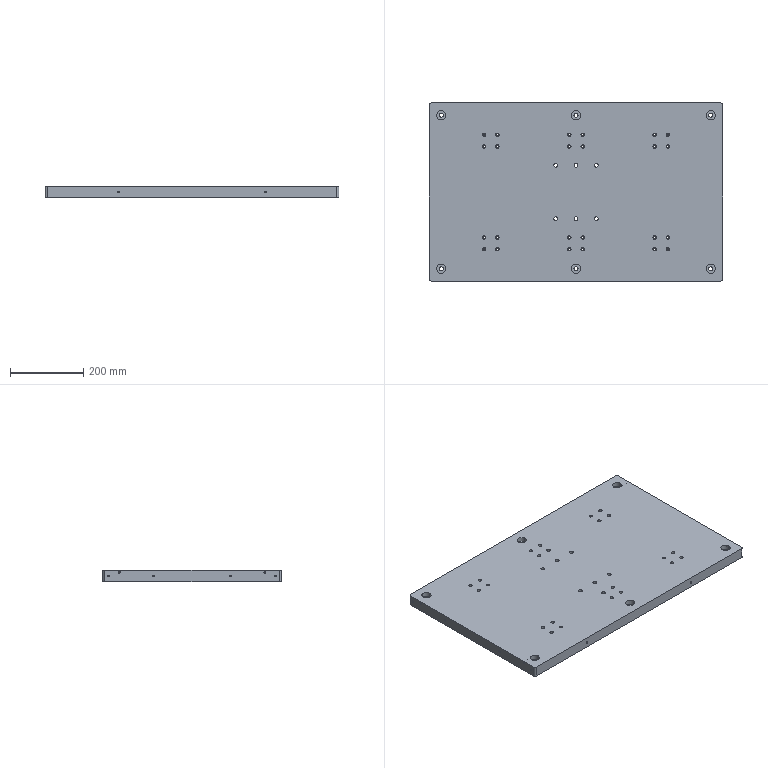NC program | Mastercam | posted with a generic post | part box 800 x 485 x 30 mm
Lines 1 to 760 of 3510:
%
O0000()
(MATERIAL - ALUMINUM MM - 2024)
( T20 | 20 FEM | H20 | XY STOCK TO LEAVE - .1 | Z STOCK TO LEAVE - .05 )
( T7 | 4 CHM | H7 )
( T1 | 11 DR | H1 | XY STOCK TO LEAVE - 0. | Z STOCK TO LEAVE - .05 )
( T14 | 10.5 DR | H14 )
( T9 | 10 FEM | H9 | XY STOCK TO LEAVE - .05 | Z STOCK TO LEAVE - .05 )
( T10 | 10 FEM | H10 | XY STOCK TO LEAVE - -.03 | Z STOCK TO LEAVE - 0. )
( T18 | 5.1 DR | H18 )
N100 G21
N110 G0 G17 G40 G49 G80 G90
( ?X )
N120 T20 M6
N130 G0 G90 G54 X-415. Y252.6 A0. S5000 M3
N140 G43 H20 Z50. M8
N150 Z1.
N160 G1 Z-.998 F600.
N170 X-395. F4000.
N180 X395.
N190 X415.
N200 Z-1.996 F600.
N210 X395. F4000.
N220 X-395.
N230 X-415.
N240 Z-2.994 F600.
N250 X-395. F4000.
N260 X395.
N270 X415.
N280 Z-3.992 F600.
N290 X395. F4000.
N300 X-395.
N310 X-415.
N320 Z-4.99 F600.
N330 X-395. F4000.
N340 X395.
N350 X415.
N360 Z-5.988 F600.
N370 X395. F4000.
N380 X-395.
N390 X-415.
N400 Z-6.986 F600.
N410 X-395. F4000.
N420 X395.
N430 X415.
N440 Z-7.984 F600.
N450 X395. F4000.
N460 X-395.
N470 X-415.
N480 Z-8.982 F600.
N490 X-395. F4000.
N500 X395.
N510 X415.
N520 Z-9.98 F600.
N530 X395. F4000.
N540 X-395.
N550 X-415.
N560 Z-10.978 F600.
N570 X-395. F4000.
N580 X395.
N590 X415.
N600 Z-11.976 F600.
N610 X395. F4000.
N620 X-395.
N630 X-415.
N640 Z-12.974 F600.
N650 X-395. F4000.
N660 X395.
N670 X415.
N680 Z-13.972 F600.
N690 X395. F4000.
N700 X-395.
N710 X-415.
N720 Z-14.97 F600.
N730 X-395. F4000.
N740 X395.
N750 X415.
N760 Z-15.968 F600.
N770 X395. F4000.
N780 X-395.
N790 X-415.
N800 Z-16.966 F600.
N810 X-395. F4000.
N820 X395.
N830 X415.
N840 Z-17.964 F600.
N850 X395. F4000.
N860 X-395.
N870 X-415.
N880 Z-18.962 F600.
N890 X-395. F4000.
N900 X395.
N910 X415.
N920 Z-19.96 F600.
N930 X395. F4000.
N940 X-395.
N950 X-415.
N960 Z-20.958 F600.
N970 X-395. F4000.
N980 X395.
N990 X415.
N1000 Z-21.956 F600.
N1010 X395. F4000.
N1020 X-395.
N1030 X-415.
N1040 Z-22.954 F600.
N1050 X-395. F4000.
N1060 X395.
N1070 X415.
N1080 Z-23.952 F600.
N1090 X395. F4000.
N1100 X-395.
N1110 X-415.
N1120 Z-24.95 F600.
N1130 X-395. F4000.
N1140 X395.
N1150 X415.
N1160 G0 Z50.
N1170 Y-252.6
N1180 Z1.
N1190 G1 Z-.998 F600.
N1200 X395. F4000.
N1210 X-395.
N1220 X-415.
N1230 Z-1.996 F600.
N1240 X-395. F4000.
N1250 X395.
N1260 X415.
N1270 Z-2.994 F600.
N1280 X395. F4000.
N1290 X-395.
N1300 X-415.
N1310 Z-3.992 F600.
N1320 X-395. F4000.
N1330 X395.
N1340 X415.
N1350 Z-4.99 F600.
N1360 X395. F4000.
N1370 X-395.
N1380 X-415.
N1390 Z-5.988 F600.
N1400 X-395. F4000.
N1410 X395.
N1420 X415.
N1430 Z-6.986 F600.
N1440 X395. F4000.
N1450 X-395.
N1460 X-415.
N1470 Z-7.984 F600.
N1480 X-395. F4000.
N1490 X395.
N1500 X415.
N1510 Z-8.982 F600.
N1520 X395. F4000.
N1530 X-395.
N1540 X-415.
N1550 Z-9.98 F600.
N1560 X-395. F4000.
N1570 X395.
N1580 X415.
N1590 Z-10.978 F600.
N1600 X395. F4000.
N1610 X-395.
N1620 X-415.
N1630 Z-11.976 F600.
N1640 X-395. F4000.
N1650 X395.
N1660 X415.
N1670 Z-12.974 F600.
N1680 X395. F4000.
N1690 X-395.
N1700 X-415.
N1710 Z-13.972 F600.
N1720 X-395. F4000.
N1730 X395.
N1740 X415.
N1750 Z-14.97 F600.
N1760 X395. F4000.
N1770 X-395.
N1780 X-415.
N1790 Z-15.968 F600.
N1800 X-395. F4000.
N1810 X395.
N1820 X415.
N1830 Z-16.966 F600.
N1840 X395. F4000.
N1850 X-395.
N1860 X-415.
N1870 Z-17.964 F600.
N1880 X-395. F4000.
N1890 X395.
N1900 X415.
N1910 Z-18.962 F600.
N1920 X395. F4000.
N1930 X-395.
N1940 X-415.
N1950 Z-19.96 F600.
N1960 X-395. F4000.
N1970 X395.
N1980 X415.
N1990 Z-20.958 F600.
N2000 X395. F4000.
N2010 X-395.
N2020 X-415.
N2030 Z-21.956 F600.
N2040 X-395. F4000.
N2050 X395.
N2060 X415.
N2070 Z-22.954 F600.
N2080 X395. F4000.
N2090 X-395.
N2100 X-415.
N2110 Z-23.952 F600.
N2120 X-395. F4000.
N2130 X395.
N2140 X415.
N2150 Z-24.95 F600.
N2160 X395. F4000.
N2170 X-395.
N2180 X-415.
N2190 G0 Z50.
N2200 Y252.53
N2210 Z1.
N2220 G1 Z-24.95 F600.
N2230 X-395. F1000.
N2240 X395.
N2250 X415.
N2260 G0 Z50.
N2270 X-415. Y252.5
N2280 Z1.
N2290 G1 Z-24.95 F600.
N2300 X-395. F1000.
N2310 X395.
N2320 X415.
N2330 G0 Z50.
N2340 Y-252.53
N2350 Z1.
N2360 G1 Z-24.95 F600.
N2370 X395. F1000.
N2380 X-395.
N2390 X-415.
N2400 G0 Z50.
N2410 X415. Y-252.5
N2420 Z1.
N2430 G1 Z-24.95 F600.
N2440 X395. F1000.
N2450 X-395.
N2460 X-415.
N2470 G0 Z50.
N2480 M5
N2490 G91 G28 Z0. M9
N2500 A0.
N2510 M01
N2520 T7 M6
N2530 G0 G90 G17 G54 X-405. Y243.15 A0. S6500 M3
N2540 G43 H7 Z50. M8
N2550 Z1.
N2560 G1 Z-.75 F600.
N2570 X-395. F1000.
N2580 X395.
N2590 X405.
N2600 G0 Z50.
N2610 Y-243.15
N2620 Z1.
N2630 G1 Z-.75 F600.
N2640 X395. F1000.
N2650 X-395.
N2660 X-405.
N2670 G0 Z50.
N2680 M5
N2690 G91 G28 Z0. M9
N2700 A0.
N2710 M01
( CCL,CY )
M00
N2720 T20 M6
N2730 G0 G90 G17 G54 X-393. Y-256.6 A0. S5000 M3
N2740 G43 H20 Z50. M8
N2750 Z1.
N2760 G1 Z-.998 F600.
N2770 Y-254.6 F4000.
N2780 G3 X-395. Y-252.6 I-2. J0.
N2790 G2 X-410.1 Y-237.5 I0. J15.1
N2800 G1 Y237.5
N2810 G2 X-395. Y252.6 I15.1 J0.
N2820 G3 X-393. Y254.6 I0. J2.
N2830 G1 Y256.6
N2840 Z-1.996 F600.
N2850 Y254.6 F4000.
N2860 G2 X-395. Y252.6 I-2. J0.
N2870 G3 X-410.1 Y237.5 I0. J-15.1
N2880 G1 Y-237.5
N2890 G3 X-395. Y-252.6 I15.1 J0.
N2900 G2 X-393. Y-254.6 I0. J-2.
N2910 G1 Y-256.6
N2920 Z-2.994 F600.
N2930 Y-254.6 F4000.
N2940 G3 X-395. Y-252.6 I-2. J0.
N2950 G2 X-410.1 Y-237.5 I0. J15.1
N2960 G1 Y237.5
N2970 G2 X-395. Y252.6 I15.1 J0.
N2980 G3 X-393. Y254.6 I0. J2.
N2990 G1 Y256.6
N3000 Z-3.992 F600.
N3010 Y254.6 F4000.
N3020 G2 X-395. Y252.6 I-2. J0.
N3030 G3 X-410.1 Y237.5 I0. J-15.1
N3040 G1 Y-237.5
N3050 G3 X-395. Y-252.6 I15.1 J0.
N3060 G2 X-393. Y-254.6 I0. J-2.
N3070 G1 Y-256.6
N3080 Z-4.99 F600.
N3090 Y-254.6 F4000.
N3100 G3 X-395. Y-252.6 I-2. J0.
N3110 G2 X-410.1 Y-237.5 I0. J15.1
N3120 G1 Y237.5
N3130 G2 X-395. Y252.6 I15.1 J0.
N3140 G3 X-393. Y254.6 I0. J2.
N3150 G1 Y256.6
N3160 Z-5.988 F600.
N3170 Y254.6 F4000.
N3180 G2 X-395. Y252.6 I-2. J0.
N3190 G3 X-410.1 Y237.5 I0. J-15.1
N3200 G1 Y-237.5
N3210 G3 X-395. Y-252.6 I15.1 J0.
N3220 G2 X-393. Y-254.6 I0. J-2.
N3230 G1 Y-256.6
N3240 Z-6.986 F600.
N3250 Y-254.6 F4000.
N3260 G3 X-395. Y-252.6 I-2. J0.
N3270 G2 X-410.1 Y-237.5 I0. J15.1
N3280 G1 Y237.5
N3290 G2 X-395. Y252.6 I15.1 J0.
N3300 G3 X-393. Y254.6 I0. J2.
N3310 G1 Y256.6
N3320 Z-7.984 F600.
N3330 Y254.6 F4000.
N3340 G2 X-395. Y252.6 I-2. J0.
N3350 G3 X-410.1 Y237.5 I0. J-15.1
N3360 G1 Y-237.5
N3370 G3 X-395. Y-252.6 I15.1 J0.
N3380 G2 X-393. Y-254.6 I0. J-2.
N3390 G1 Y-256.6
N3400 Z-8.982 F600.
N3410 Y-254.6 F4000.
N3420 G3 X-395. Y-252.6 I-2. J0.
N3430 G2 X-410.1 Y-237.5 I0. J15.1
N3440 G1 Y237.5
N3450 G2 X-395. Y252.6 I15.1 J0.
N3460 G3 X-393. Y254.6 I0. J2.
N3470 G1 Y256.6
N3480 Z-9.98 F600.
N3490 Y254.6 F4000.
N3500 G2 X-395. Y252.6 I-2. J0.
N3510 G3 X-410.1 Y237.5 I0. J-15.1
N3520 G1 Y-237.5
N3530 G3 X-395. Y-252.6 I15.1 J0.
N3540 G2 X-393. Y-254.6 I0. J-2.
N3550 G1 Y-256.6
N3560 Z-10.978 F600.
N3570 Y-254.6 F4000.
N3580 G3 X-395. Y-252.6 I-2. J0.
N3590 G2 X-410.1 Y-237.5 I0. J15.1
N3600 G1 Y237.5
N3610 G2 X-395. Y252.6 I15.1 J0.
N3620 G3 X-393. Y254.6 I0. J2.
N3630 G1 Y256.6
N3640 Z-11.976 F600.
N3650 Y254.6 F4000.
N3660 G2 X-395. Y252.6 I-2. J0.
N3670 G3 X-410.1 Y237.5 I0. J-15.1
N3680 G1 Y-237.5
N3690 G3 X-395. Y-252.6 I15.1 J0.
N3700 G2 X-393. Y-254.6 I0. J-2.
N3710 G1 Y-256.6
N3720 Z-12.974 F600.
N3730 Y-254.6 F4000.
N3740 G3 X-395. Y-252.6 I-2. J0.
N3750 G2 X-410.1 Y-237.5 I0. J15.1
N3760 G1 Y237.5
N3770 G2 X-395. Y252.6 I15.1 J0.
N3780 G3 X-393. Y254.6 I0. J2.
N3790 G1 Y256.6
N3800 Z-13.972 F600.
N3810 Y254.6 F4000.
N3820 G2 X-395. Y252.6 I-2. J0.
N3830 G3 X-410.1 Y237.5 I0. J-15.1
N3840 G1 Y-237.5
N3850 G3 X-395. Y-252.6 I15.1 J0.
N3860 G2 X-393. Y-254.6 I0. J-2.
N3870 G1 Y-256.6
N3880 Z-14.97 F600.
N3890 Y-254.6 F4000.
N3900 G3 X-395. Y-252.6 I-2. J0.
N3910 G2 X-410.1 Y-237.5 I0. J15.1
N3920 G1 Y237.5
N3930 G2 X-395. Y252.6 I15.1 J0.
N3940 G3 X-393. Y254.6 I0. J2.
N3950 G1 Y256.6
N3960 Z-15.968 F600.
N3970 Y254.6 F4000.
N3980 G2 X-395. Y252.6 I-2. J0.
N3990 G3 X-410.1 Y237.5 I0. J-15.1
N4000 G1 Y-237.5
N4010 G3 X-395. Y-252.6 I15.1 J0.
N4020 G2 X-393. Y-254.6 I0. J-2.
N4030 G1 Y-256.6
N4040 Z-16.966 F600.
N4050 Y-254.6 F4000.
N4060 G3 X-395. Y-252.6 I-2. J0.
N4070 G2 X-410.1 Y-237.5 I0. J15.1
N4080 G1 Y237.5
N4090 G2 X-395. Y252.6 I15.1 J0.
N4100 G3 X-393. Y254.6 I0. J2.
N4110 G1 Y256.6
N4120 Z-17.964 F600.
N4130 Y254.6 F4000.
N4140 G2 X-395. Y252.6 I-2. J0.
N4150 G3 X-410.1 Y237.5 I0. J-15.1
N4160 G1 Y-237.5
N4170 G3 X-395. Y-252.6 I15.1 J0.
N4180 G2 X-393. Y-254.6 I0. J-2.
N4190 G1 Y-256.6
N4200 Z-18.962 F600.
N4210 Y-254.6 F4000.
N4220 G3 X-395. Y-252.6 I-2. J0.
N4230 G2 X-410.1 Y-237.5 I0. J15.1
N4240 G1 Y237.5
N4250 G2 X-395. Y252.6 I15.1 J0.
N4260 G3 X-393. Y254.6 I0. J2.
N4270 G1 Y256.6
N4280 Z-19.96 F600.
N4290 Y254.6 F4000.
N4300 G2 X-395. Y252.6 I-2. J0.
N4310 G3 X-410.1 Y237.5 I0. J-15.1
N4320 G1 Y-237.5
N4330 G3 X-395. Y-252.6 I15.1 J0.
N4340 G2 X-393. Y-254.6 I0. J-2.
N4350 G1 Y-256.6
N4360 Z-20.958 F600.
N4370 Y-254.6 F4000.
N4380 G3 X-395. Y-252.6 I-2. J0.
N4390 G2 X-410.1 Y-237.5 I0. J15.1
N4400 G1 Y237.5
N4410 G2 X-395. Y252.6 I15.1 J0.
N4420 G3 X-393. Y254.6 I0. J2.
N4430 G1 Y256.6
N4440 Z-21.956 F600.
N4450 Y254.6 F4000.
N4460 G2 X-395. Y252.6 I-2. J0.
N4470 G3 X-410.1 Y237.5 I0. J-15.1
N4480 G1 Y-237.5
N4490 G3 X-395. Y-252.6 I15.1 J0.
N4500 G2 X-393. Y-254.6 I0. J-2.
N4510 G1 Y-256.6
N4520 Z-22.954 F600.
N4530 Y-254.6 F4000.
N4540 G3 X-395. Y-252.6 I-2. J0.
N4550 G2 X-410.1 Y-237.5 I0. J15.1
N4560 G1 Y237.5
N4570 G2 X-395. Y252.6 I15.1 J0.
N4580 G3 X-393. Y254.6 I0. J2.
N4590 G1 Y256.6
N4600 Z-23.952 F600.
N4610 Y254.6 F4000.
N4620 G2 X-395. Y252.6 I-2. J0.
N4630 G3 X-410.1 Y237.5 I0. J-15.1
N4640 G1 Y-237.5
N4650 G3 X-395. Y-252.6 I15.1 J0.
N4660 G2 X-393. Y-254.6 I0. J-2.
N4670 G1 Y-256.6
N4680 Z-24.95 F600.
N4690 Y-254.6 F4000.
N4700 G3 X-395. Y-252.6 I-2. J0.
N4710 G2 X-410.1 Y-237.5 I0. J15.1
N4720 G1 Y237.5
N4730 G2 X-395. Y252.6 I15.1 J0.
N4740 G3 X-393. Y254.6 I0. J2.
N4750 G1 Y256.6
N4760 G0 Z50.
N4770 X393.
N4780 Z1.
N4790 G1 Z-.998 F600.
N4800 Y254.6 F4000.
N4810 G3 X395. Y252.6 I2. J0.
N4820 G2 X410.1 Y237.5 I0. J-15.1
N4830 G1 Y-237.5
N4840 G2 X395. Y-252.6 I-15.1 J0.
N4850 G3 X393. Y-254.6 I0. J-2.
N4860 G1 Y-256.6
N4870 Z-1.996 F600.
N4880 Y-254.6 F4000.
N4890 G2 X395. Y-252.6 I2. J0.
N4900 G3 X410.1 Y-237.5 I0. J15.1
N4910 G1 Y237.5
N4920 G3 X395. Y252.6 I-15.1 J0.
N4930 G2 X393. Y254.6 I0. J2.
N4940 G1 Y256.6
N4950 Z-2.994 F600.
N4960 Y254.6 F4000.
N4970 G3 X395. Y252.6 I2. J0.
N4980 G2 X410.1 Y237.5 I0. J-15.1
N4990 G1 Y-237.5
N5000 G2 X395. Y-252.6 I-15.1 J0.
N5010 G3 X393. Y-254.6 I0. J-2.
N5020 G1 Y-256.6
N5030 Z-3.992 F600.
N5040 Y-254.6 F4000.
N5050 G2 X395. Y-252.6 I2. J0.
N5060 G3 X410.1 Y-237.5 I0. J15.1
N5070 G1 Y237.5
N5080 G3 X395. Y252.6 I-15.1 J0.
N5090 G2 X393. Y254.6 I0. J2.
N5100 G1 Y256.6
N5110 Z-4.99 F600.
N5120 Y254.6 F4000.
N5130 G3 X395. Y252.6 I2. J0.
N5140 G2 X410.1 Y237.5 I0. J-15.1
N5150 G1 Y-237.5
N5160 G2 X395. Y-252.6 I-15.1 J0.
N5170 G3 X393. Y-254.6 I0. J-2.
N5180 G1 Y-256.6
N5190 Z-5.988 F600.
N5200 Y-254.6 F4000.
N5210 G2 X395. Y-252.6 I2. J0.
N5220 G3 X410.1 Y-237.5 I0. J15.1
N5230 G1 Y237.5
N5240 G3 X395. Y252.6 I-15.1 J0.
N5250 G2 X393. Y254.6 I0. J2.
N5260 G1 Y256.6
N5270 Z-6.986 F600.
N5280 Y254.6 F4000.
N5290 G3 X395. Y252.6 I2. J0.
N5300 G2 X410.1 Y237.5 I0. J-15.1
N5310 G1 Y-237.5
N5320 G2 X395. Y-252.6 I-15.1 J0.
N5330 G3 X393. Y-254.6 I0. J-2.
N5340 G1 Y-256.6
N5350 Z-7.984 F600.
N5360 Y-254.6 F4000.
N5370 G2 X395. Y-252.6 I2. J0.
N5380 G3 X410.1 Y-237.5 I0. J15.1
N5390 G1 Y237.5
N5400 G3 X395. Y252.6 I-15.1 J0.
N5410 G2 X393. Y254.6 I0. J2.
N5420 G1 Y256.6
N5430 Z-8.982 F600.
N5440 Y254.6 F4000.
N5450 G3 X395. Y252.6 I2. J0.
N5460 G2 X410.1 Y237.5 I0. J-15.1
N5470 G1 Y-237.5
N5480 G2 X395. Y-252.6 I-15.1 J0.
N5490 G3 X393. Y-254.6 I0. J-2.
N5500 G1 Y-256.6
N5510 Z-9.98 F600.
N5520 Y-254.6 F4000.
N5530 G2 X395. Y-252.6 I2. J0.
N5540 G3 X410.1 Y-237.5 I0. J15.1
N5550 G1 Y237.5
N5560 G3 X395. Y252.6 I-15.1 J0.
N5570 G2 X393. Y254.6 I0. J2.
N5580 G1 Y256.6
N5590 Z-10.978 F600.
N5600 Y254.6 F4000.
N5610 G3 X395. Y252.6 I2. J0.
N5620 G2 X410.1 Y237.5 I0. J-15.1
N5630 G1 Y-237.5
N5640 G2 X395. Y-252.6 I-15.1 J0.
N5650 G3 X393. Y-254.6 I0. J-2.
N5660 G1 Y-256.6
N5670 Z-11.976 F600.
N5680 Y-254.6 F4000.
N5690 G2 X395. Y-252.6 I2. J0.
N5700 G3 X410.1 Y-237.5 I0. J15.1
N5710 G1 Y237.5
N5720 G3 X395. Y252.6 I-15.1 J0.
N5730 G2 X393. Y254.6 I0. J2.
N5740 G1 Y256.6
N5750 Z-12.974 F600.
N5760 Y254.6 F4000.
N5770 G3 X395. Y252.6 I2. J0.
N5780 G2 X410.1 Y237.5 I0. J-15.1
N5790 G1 Y-237.5
N5800 G2 X395. Y-252.6 I-15.1 J0.
N5810 G3 X393. Y-254.6 I0. J-2.
N5820 G1 Y-256.6
N5830 Z-13.972 F600.
N5840 Y-254.6 F4000.
N5850 G2 X395. Y-252.6 I2. J0.
N5860 G3 X410.1 Y-237.5 I0. J15.1
N5870 G1 Y237.5
N5880 G3 X395. Y252.6 I-15.1 J0.
N5890 G2 X393. Y254.6 I0. J2.
N5900 G1 Y256.6
N5910 Z-14.97 F600.
N5920 Y254.6 F4000.
N5930 G3 X395. Y252.6 I2. J0.
N5940 G2 X410.1 Y237.5 I0. J-15.1
N5950 G1 Y-237.5
N5960 G2 X395. Y-252.6 I-15.1 J0.
N5970 G3 X393. Y-254.6 I0. J-2.
N5980 G1 Y-256.6
N5990 Z-15.968 F600.
N6000 Y-254.6 F4000.
N6010 G2 X395. Y-252.6 I2. J0.
N6020 G3 X410.1 Y-237.5 I0. J15.1
N6030 G1 Y237.5
N6040 G3 X395. Y252.6 I-15.1 J0.
N6050 G2 X393. Y254.6 I0. J2.
N6060 G1 Y256.6
N6070 Z-16.966 F600.
N6080 Y254.6 F4000.
N6090 G3 X395. Y252.6 I2. J0.
N6100 G2 X410.1 Y237.5 I0. J-15.1
N6110 G1 Y-237.5
N6120 G2 X395. Y-252.6 I-15.1 J0.
N6130 G3 X393. Y-254.6 I0. J-2.
N6140 G1 Y-256.6
N6150 Z-17.964 F600.
N6160 Y-254.6 F4000.
N6170 G2 X395. Y-252.6 I2. J0.
N6180 G3 X410.1 Y-237.5 I0. J15.1
N6190 G1 Y237.5
N6200 G3 X395. Y252.6 I-15.1 J0.
N6210 G2 X393. Y254.6 I0. J2.
N6220 G1 Y256.6
N6230 Z-18.962 F600.
N6240 Y254.6 F4000.
N6250 G3 X395. Y252.6 I2. J0.
N6260 G2 X410.1 Y237.5 I0. J-15.1
N6270 G1 Y-237.5
N6280 G2 X395. Y-252.6 I-15.1 J0.
N6290 G3 X393. Y-254.6 I0. J-2.
N6300 G1 Y-256.6
N6310 Z-19.96 F600.
N6320 Y-254.6 F4000.
N6330 G2 X395. Y-252.6 I2. J0.
N6340 G3 X410.1 Y-237.5 I0. J15.1
N6350 G1 Y237.5
N6360 G3 X395. Y252.6 I-15.1 J0.
N6370 G2 X393. Y254.6 I0. J2.
N6380 G1 Y256.6
N6390 Z-20.958 F600.
N6400 Y254.6 F4000.
N6410 G3 X395. Y252.6 I2. J0.
N6420 G2 X410.1 Y237.5 I0. J-15.1
N6430 G1 Y-237.5
N6440 G2 X395. Y-252.6 I-15.1 J0.
N6450 G3 X393. Y-254.6 I0. J-2.
N6460 G1 Y-256.6
N6470 Z-21.956 F600.
N6480 Y-254.6 F4000.
N6490 G2 X395. Y-252.6 I2. J0.
N6500 G3 X410.1 Y-237.5 I0. J15.1
N6510 G1 Y237.5
N6520 G3 X395. Y252.6 I-15.1 J0.
N6530 G2 X393. Y254.6 I0. J2.
N6540 G1 Y256.6
N6550 Z-22.954 F600.
N6560 Y254.6 F4000.
N6570 G3 X395. Y252.6 I2. J0.
N6580 G2 X410.1 Y237.5 I0. J-15.1
N6590 G1 Y-237.5
N6600 G2 X395. Y-252.6 I-15.1 J0.
N6610 G3 X393. Y-254.6 I0. J-2.
N6620 G1 Y-256.6
N6630 Z-23.952 F600.
N6640 Y-254.6 F4000.
N6650 G2 X395. Y-252.6 I2. J0.
N6660 G3 X410.1 Y-237.5 I0. J15.1
N6670 G1 Y237.5
N6680 G3 X395. Y252.6 I-15.1 J0.
N6690 G2 X393. Y254.6 I0. J2.
N6700 G1 Y256.6
N6710 Z-24.95 F600.
N6720 Y254.6 F4000.
N6730 G3 X395. Y252.6 I2. J0.
N6740 G2 X410.1 Y237.5 I0. J-15.1
N6750 G1 Y-237.5
N6760 G2 X395. Y-252.6 I-15.1 J0.
N6770 G3 X393. Y-254.6 I0. J-2.
N6780 G1 Y-256.6
N6790 G0 Z50.
N6800 X-393. Y-256.53
N6810 Z1.
N6820 G1 Z-24.95 F600.
N6830 Y-254.53 F1000.
N6840 G3 X-395. Y-252.53 I-2. J0.
N6850 G2 X-410.03 Y-237.5 I0. J15.03
N6860 G1 Y237.5
N6870 G2 X-395. Y252.53 I15.03 J0.
N6880 G3 X-393. Y254.53 I0. J2.
N6890 G1 Y256.53
N6900 G0 Z50.
N6910 Y-256.5
N6920 Z1.
N6930 G1 Z-24.95 F600.
N6940 Y-254.5 F1000.
N6950 G3 X-395. Y-252.5 I-2. J0.
N6960 G2 X-410. Y-237.5 I0. J15.
N6970 G1 Y237.5
N6980 G2 X-395. Y252.5 I15. J0.
N6990 G3 X-393. Y254.5 I0. J2.
N7000 G1 Y256.5
N7010 G0 Z50.
N7020 X393. Y256.53
N7030 Z1.
N7040 G1 Z-24.95 F600.
N7050 Y254.53 F1000.
N7060 G3 X395. Y252.53 I2. J0.
N7070 G2 X410.03 Y237.5 I0. J-15.03
N7080 G1 Y-237.5
N7090 G2 X395. Y-252.53 I-15.03 J0.
N7100 G3 X393. Y-254.53 I0. J-2.
N7110 G1 Y-256.53
N7120 G0 Z50.
N7130 Y256.5
N7140 Z1.
N7150 G1 Z-24.95 F600.
N7160 Y254.5 F1000.
N7170 G3 X395. Y252.5 I2. J0.
N7180 G2 X410. Y237.5 I0. J-15.
N7190 G1 Y-237.5
N7200 G2 X395. Y-252.5 I-15. J0.
N7210 G3 X393. Y-254.5 I0. J-2.
N7220 G1 Y-256.5
N7230 G0 Z50.
N7240 M5
N7250 G91 G28 Z0. M9
N7260 A0.
N7270 M01
N7280 T7 M6
N7290 G0 G90 G17 G54 X-394.6 Y-243.95 A0. S6500 M3
N7300 G43 H7 Z50. M8
N7310 Z1.
N7320 G1 Z-.75 F600.
N7330 Y-243.55 F1000.
N7340 G3 X-395. Y-243.15 I-.4 J0.
N7350 G2 X-400.65 Y-237.5 I0. J5.65
N7360 G1 Y237.5
N7370 G2 X-395. Y243.15 I5.65 J0.
N7380 G3 X-394.6 Y243.55 I0. J.4
N7390 G1 Y243.95
N7400 G0 Z50.
N7410 X394.6
N7420 Z1.
N7430 G1 Z-.75 F600.
N7440 Y243.55 F1000.
N7450 G3 X395. Y243.15 I.4 J0.
N7460 G2 X400.65 Y237.5 I0. J-5.65
N7470 G1 Y-237.5
N7480 G2 X395. Y-243.15 I-5.65 J0.
N7490 G3 X394.6 Y-243.55 I0. J-.4
N7500 G1 Y-243.95
N7510 G0 Z50.
N7520 M5
N7530 G91 G28 Z0. M9
N7540 A0.
N7550 M01
M00